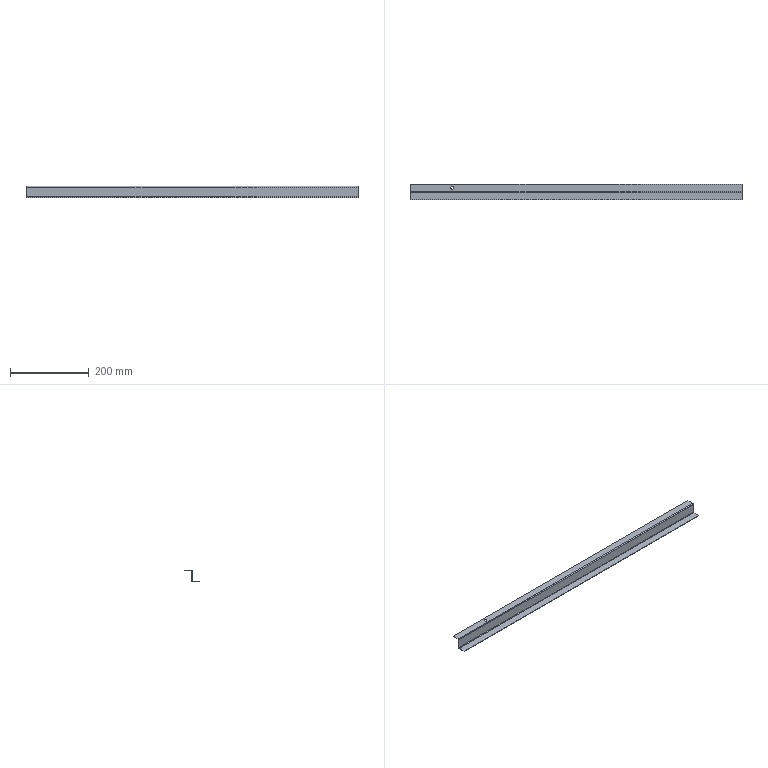Part | SolidWorks | features EdgeFlange 2, FlatPattern 1, HoleWzd 1, SMBaseFlange 1, SheetMetal 1 | 1 solid | 24 faces | box 843 x 38.8 x 28.5 mm | volume 65431 mm3 | plane 18 | cylinder 6 | commonest cylinder face diameters 2 x2 4.4 x2 7 x2
STEP:
#1=CARTESIAN_POINT('',(-310.891,19.773,26.1));
#2=VERTEX_POINT('',#1);
#3=CARTESIAN_POINT('',(-317.891,19.773,26.1));
#4=VERTEX_POINT('',#3);
#5=CARTESIAN_POINT('',(-314.391,19.773,26.1));
#6=DIRECTION('',(0.,0.,-1.));
#7=DIRECTION('',(-1.,0.,0.));
#8=AXIS2_PLACEMENT_3D('',#5,#6,#7);
#9=CIRCLE('',#8,3.5);
#10=EDGE_CURVE('',#2,#4,#9,.T.);
#11=ORIENTED_EDGE('',*,*,#10,.T.);
#12=CARTESIAN_POINT('',(-317.891,19.773,27.3));
#13=VERTEX_POINT('',#12);
#14=CARTESIAN_POINT('',(-317.891,19.773,27.3));
#15=DIRECTION('',(0.,0.,1.));
#16=VECTOR('',#15,1000.);
#17=LINE('',#14,#16);
#18=EDGE_CURVE('',#4,#13,#17,.T.);
#19=ORIENTED_EDGE('',*,*,#18,.T.);
#20=CARTESIAN_POINT('',(-310.891,19.773,27.3));
#21=VERTEX_POINT('',#20);
#22=CARTESIAN_POINT('',(-314.391,19.773,27.3));
#23=DIRECTION('',(0.,0.,1.));
#24=DIRECTION('',(1.,0.,0.));
#25=AXIS2_PLACEMENT_3D('',#22,#23,#24);
#26=CIRCLE('',#25,3.5);
#27=EDGE_CURVE('',#13,#21,#26,.T.);
#28=ORIENTED_EDGE('',*,*,#27,.T.);
#29=CARTESIAN_POINT('',(-310.891,19.773,27.3));
#30=DIRECTION('',(0.,0.,1.));
#31=VECTOR('',#30,1000.);
#32=LINE('',#29,#31);
#33=EDGE_CURVE('',#2,#21,#32,.T.);
#34=ORIENTED_EDGE('',*,*,#33,.F.);
#35=EDGE_LOOP('',(#11,#19,#28,#34));
#36=FACE_OUTER_BOUND('',#35,.T.);
#37=CARTESIAN_POINT('',(-314.391,19.773,27.3));
#38=DIRECTION('',(0.,0.,1.));
#39=DIRECTION('',(1.,0.,0.));
#40=AXIS2_PLACEMENT_3D('',#37,#38,#39);
#41=CYLINDRICAL_SURFACE('',#40,3.5);
#42=ADVANCED_FACE('',(#36),#41,.F.);
#43=CARTESIAN_POINT('',(421.5,10.,25.1));
#44=VERTEX_POINT('',#43);
#45=CARTESIAN_POINT('',(421.5,8.8,25.1));
#46=VERTEX_POINT('',#45);
#47=CARTESIAN_POINT('',(421.5,10.,25.1));
#48=DIRECTION('',(0.,-1.,0.));
#49=VECTOR('',#48,1000.);
#50=LINE('',#47,#49);
#51=EDGE_CURVE('',#44,#46,#50,.T.);
#52=ORIENTED_EDGE('',*,*,#51,.T.);
#53=CARTESIAN_POINT('',(421.5,8.8,1.));
#54=VERTEX_POINT('',#53);
#55=CARTESIAN_POINT('',(421.5,8.8,0.));
#56=DIRECTION('',(0.,0.,-1.));
#57=VECTOR('',#56,1000.);
#58=LINE('',#55,#57);
#59=EDGE_CURVE('',#46,#54,#58,.T.);
#60=ORIENTED_EDGE('',*,*,#59,.T.);
#61=CARTESIAN_POINT('',(421.5,10.,1.));
#62=VERTEX_POINT('',#61);
#63=CARTESIAN_POINT('',(421.5,10.,1.));
#64=DIRECTION('',(0.,1.,0.));
#65=VECTOR('',#64,1000.);
#66=LINE('',#63,#65);
#67=EDGE_CURVE('',#54,#62,#66,.T.);
#68=ORIENTED_EDGE('',*,*,#67,.T.);
#69=CARTESIAN_POINT('',(421.5,10.,0.));
#70=DIRECTION('',(0.,0.,-1.));
#71=VECTOR('',#70,1000.);
#72=LINE('',#69,#71);
#73=EDGE_CURVE('',#44,#62,#72,.T.);
#74=ORIENTED_EDGE('',*,*,#73,.F.);
#75=EDGE_LOOP('',(#52,#60,#68,#74));
#76=FACE_OUTER_BOUND('',#75,.T.);
#77=CARTESIAN_POINT('',(421.5,10.,0.));
#78=DIRECTION('',(-1.,0.,0.));
#79=DIRECTION('',(0.,0.,1.));
#80=AXIS2_PLACEMENT_3D('',#77,#78,#79);
#81=PLANE('',#80);
#82=ADVANCED_FACE('',(#76),#81,.F.);
#83=CARTESIAN_POINT('',(-421.5,10.,25.1));
#84=VERTEX_POINT('',#83);
#85=CARTESIAN_POINT('',(-421.5,8.8,25.1));
#86=VERTEX_POINT('',#85);
#87=CARTESIAN_POINT('',(-421.5,10.,25.1));
#88=DIRECTION('',(0.,-1.,0.));
#89=VECTOR('',#88,1000.);
#90=LINE('',#87,#89);
#91=EDGE_CURVE('',#84,#86,#90,.T.);
#92=ORIENTED_EDGE('',*,*,#91,.F.);
#93=CARTESIAN_POINT('',(-421.5,10.,1.));
#94=VERTEX_POINT('',#93);
#95=CARTESIAN_POINT('',(-421.5,10.,0.));
#96=DIRECTION('',(0.,0.,1.));
#97=VECTOR('',#96,1000.);
#98=LINE('',#95,#97);
#99=EDGE_CURVE('',#94,#84,#98,.T.);
#100=ORIENTED_EDGE('',*,*,#99,.F.);
#101=CARTESIAN_POINT('',(-421.5,8.8,1.));
#102=VERTEX_POINT('',#101);
#103=CARTESIAN_POINT('',(-421.5,8.8,1.));
#104=DIRECTION('',(0.,1.,0.));
#105=VECTOR('',#104,1000.);
#106=LINE('',#103,#105);
#107=EDGE_CURVE('',#102,#94,#106,.T.);
#108=ORIENTED_EDGE('',*,*,#107,.F.);
#109=CARTESIAN_POINT('',(-421.5,8.8,27.3));
#110=DIRECTION('',(0.,0.,1.));
#111=VECTOR('',#110,1000.);
#112=LINE('',#109,#111);
#113=EDGE_CURVE('',#102,#86,#112,.T.);
#114=ORIENTED_EDGE('',*,*,#113,.T.);
#115=EDGE_LOOP('',(#92,#100,#108,#114));
#116=FACE_OUTER_BOUND('',#115,.T.);
#117=CARTESIAN_POINT('',(-421.5,10.,27.3));
#118=DIRECTION('',(1.,0.,0.));
#119=DIRECTION('',(0.,0.,-1.));
#120=AXIS2_PLACEMENT_3D('',#117,#118,#119);
#121=PLANE('',#120);
#122=ADVANCED_FACE('',(#116),#121,.F.);
#123=CARTESIAN_POINT('',(421.5,10.,25.1));
#124=DIRECTION('',(-1.,0.,0.));
#125=VECTOR('',#124,1000.);
#126=LINE('',#123,#125);
#127=EDGE_CURVE('',#44,#84,#126,.T.);
#128=ORIENTED_EDGE('',*,*,#127,.F.);
#129=ORIENTED_EDGE('',*,*,#73,.T.);
#130=CARTESIAN_POINT('',(421.5,10.,1.));
#131=DIRECTION('',(1.,0.,0.));
#132=VECTOR('',#131,1000.);
#133=LINE('',#130,#132);
#134=EDGE_CURVE('',#94,#62,#133,.T.);
#135=ORIENTED_EDGE('',*,*,#134,.F.);
#136=ORIENTED_EDGE('',*,*,#99,.T.);
#137=EDGE_LOOP('',(#128,#129,#135,#136));
#138=FACE_OUTER_BOUND('',#137,.T.);
#139=CARTESIAN_POINT('',(0.,10.,0.));
#140=DIRECTION('',(0.,-1.,0.));
#141=DIRECTION('',(0.,0.,-1.));
#142=AXIS2_PLACEMENT_3D('',#139,#140,#141);
#143=PLANE('',#142);
#144=ADVANCED_FACE('',(#138),#143,.F.);
#145=ORIENTED_EDGE('',*,*,#59,.F.);
#146=CARTESIAN_POINT('',(421.5,8.8,25.1));
#147=DIRECTION('',(-1.,0.,0.));
#148=VECTOR('',#147,1000.);
#149=LINE('',#146,#148);
#150=EDGE_CURVE('',#46,#86,#149,.T.);
#151=ORIENTED_EDGE('',*,*,#150,.T.);
#152=ORIENTED_EDGE('',*,*,#113,.F.);
#153=CARTESIAN_POINT('',(421.5,8.8,1.));
#154=DIRECTION('',(-1.,0.,0.));
#155=VECTOR('',#154,1000.);
#156=LINE('',#153,#155);
#157=EDGE_CURVE('',#54,#102,#156,.T.);
#158=ORIENTED_EDGE('',*,*,#157,.F.);
#159=EDGE_LOOP('',(#145,#151,#152,#158));
#160=FACE_OUTER_BOUND('',#159,.T.);
#161=CARTESIAN_POINT('',(0.,8.8,0.));
#162=DIRECTION('',(0.,-1.,0.));
#163=DIRECTION('',(0.,0.,-1.));
#164=AXIS2_PLACEMENT_3D('',#161,#162,#163);
#165=PLANE('',#164);
#166=ADVANCED_FACE('',(#160),#165,.T.);
#167=CARTESIAN_POINT('',(-421.5,7.8,0.));
#168=VERTEX_POINT('',#167);
#169=CARTESIAN_POINT('',(-421.5,-10.,0.));
#170=VERTEX_POINT('',#169);
#171=CARTESIAN_POINT('',(-421.5,10.,0.));
#172=DIRECTION('',(0.,-1.,0.));
#173=VECTOR('',#172,1000.);
#174=LINE('',#171,#173);
#175=EDGE_CURVE('',#168,#170,#174,.T.);
#176=ORIENTED_EDGE('',*,*,#175,.F.);
#177=CARTESIAN_POINT('',(-421.5,7.8,-1.2));
#178=VERTEX_POINT('',#177);
#179=CARTESIAN_POINT('',(-421.5,7.8,0.));
#180=DIRECTION('',(0.,0.,-1.));
#181=VECTOR('',#180,1000.);
#182=LINE('',#179,#181);
#183=EDGE_CURVE('',#168,#178,#182,.T.);
#184=ORIENTED_EDGE('',*,*,#183,.T.);
#185=CARTESIAN_POINT('',(-421.5,-10.,-1.2));
#186=VERTEX_POINT('',#185);
#187=CARTESIAN_POINT('',(-421.5,10.,-1.2));
#188=DIRECTION('',(0.,-1.,0.));
#189=VECTOR('',#188,1000.);
#190=LINE('',#187,#189);
#191=EDGE_CURVE('',#178,#186,#190,.T.);
#192=ORIENTED_EDGE('',*,*,#191,.T.);
#193=CARTESIAN_POINT('',(-421.5,-10.,-1.2));
#194=DIRECTION('',(0.,0.,1.));
#195=VECTOR('',#194,1000.);
#196=LINE('',#193,#195);
#197=EDGE_CURVE('',#186,#170,#196,.T.);
#198=ORIENTED_EDGE('',*,*,#197,.T.);
#199=EDGE_LOOP('',(#176,#184,#192,#198));
#200=FACE_OUTER_BOUND('',#199,.T.);
#201=CARTESIAN_POINT('',(-421.5,10.,-1.2));
#202=DIRECTION('',(-1.,0.,0.));
#203=DIRECTION('',(0.,0.,1.));
#204=AXIS2_PLACEMENT_3D('',#201,#202,#203);
#205=PLANE('',#204);
#206=ADVANCED_FACE('',(#200),#205,.T.);
#207=CARTESIAN_POINT('',(421.5,7.8,-1.2));
#208=VERTEX_POINT('',#207);
#209=CARTESIAN_POINT('',(-421.5,7.8,-1.2));
#210=DIRECTION('',(1.,0.,0.));
#211=VECTOR('',#210,1000.);
#212=LINE('',#209,#211);
#213=EDGE_CURVE('',#178,#208,#212,.T.);
#214=ORIENTED_EDGE('',*,*,#213,.T.);
#215=CARTESIAN_POINT('',(421.5,-10.,-1.2));
#216=VERTEX_POINT('',#215);
#217=CARTESIAN_POINT('',(421.5,10.,-1.2));
#218=DIRECTION('',(0.,1.,0.));
#219=VECTOR('',#218,1000.);
#220=LINE('',#217,#219);
#221=EDGE_CURVE('',#216,#208,#220,.T.);
#222=ORIENTED_EDGE('',*,*,#221,.F.);
#223=CARTESIAN_POINT('',(-421.5,-10.,-1.2));
#224=DIRECTION('',(1.,0.,0.));
#225=VECTOR('',#224,1000.);
#226=LINE('',#223,#225);
#227=EDGE_CURVE('',#186,#216,#226,.T.);
#228=ORIENTED_EDGE('',*,*,#227,.F.);
#229=ORIENTED_EDGE('',*,*,#191,.F.);
#230=EDGE_LOOP('',(#214,#222,#228,#229));
#231=FACE_OUTER_BOUND('',#230,.T.);
#232=CARTESIAN_POINT('',(0.,0.,-1.2));
#233=DIRECTION('',(0.,0.,1.));
#234=DIRECTION('',(1.,0.,0.));
#235=AXIS2_PLACEMENT_3D('',#232,#233,#234);
#236=PLANE('',#235);
#237=ADVANCED_FACE('',(#231),#236,.F.);
#238=CARTESIAN_POINT('',(421.5,-10.,0.));
#239=VERTEX_POINT('',#238);
#240=CARTESIAN_POINT('',(421.5,7.8,0.));
#241=VERTEX_POINT('',#240);
#242=CARTESIAN_POINT('',(421.5,10.,0.));
#243=DIRECTION('',(0.,1.,0.));
#244=VECTOR('',#243,1000.);
#245=LINE('',#242,#244);
#246=EDGE_CURVE('',#239,#241,#245,.T.);
#247=ORIENTED_EDGE('',*,*,#246,.T.);
#248=CARTESIAN_POINT('',(-421.5,7.8,0.));
#249=DIRECTION('',(1.,0.,0.));
#250=VECTOR('',#249,1000.);
#251=LINE('',#248,#250);
#252=EDGE_CURVE('',#168,#241,#251,.T.);
#253=ORIENTED_EDGE('',*,*,#252,.F.);
#254=ORIENTED_EDGE('',*,*,#175,.T.);
#255=CARTESIAN_POINT('',(-421.5,-10.,0.));
#256=DIRECTION('',(1.,0.,0.));
#257=VECTOR('',#256,1000.);
#258=LINE('',#255,#257);
#259=EDGE_CURVE('',#170,#239,#258,.T.);
#260=ORIENTED_EDGE('',*,*,#259,.T.);
#261=EDGE_LOOP('',(#247,#253,#254,#260));
#262=FACE_OUTER_BOUND('',#261,.T.);
#263=CARTESIAN_POINT('',(0.,0.,0.));
#264=DIRECTION('',(0.,0.,1.));
#265=DIRECTION('',(1.,0.,0.));
#266=AXIS2_PLACEMENT_3D('',#263,#264,#265);
#267=PLANE('',#266);
#268=ADVANCED_FACE('',(#262),#267,.T.);
#269=CARTESIAN_POINT('',(421.5,7.8,0.));
#270=DIRECTION('',(0.,0.,-1.));
#271=VECTOR('',#270,1000.);
#272=LINE('',#269,#271);
#273=EDGE_CURVE('',#241,#208,#272,.T.);
#274=ORIENTED_EDGE('',*,*,#273,.F.);
#275=ORIENTED_EDGE('',*,*,#246,.F.);
#276=CARTESIAN_POINT('',(421.5,-10.,-1.2));
#277=DIRECTION('',(0.,0.,1.));
#278=VECTOR('',#277,1000.);
#279=LINE('',#276,#278);
#280=EDGE_CURVE('',#216,#239,#279,.T.);
#281=ORIENTED_EDGE('',*,*,#280,.F.);
#282=ORIENTED_EDGE('',*,*,#221,.T.);
#283=EDGE_LOOP('',(#274,#275,#281,#282));
#284=FACE_OUTER_BOUND('',#283,.T.);
#285=CARTESIAN_POINT('',(421.5,10.,-1.2));
#286=DIRECTION('',(1.,0.,0.));
#287=DIRECTION('',(0.,0.,-1.));
#288=AXIS2_PLACEMENT_3D('',#285,#286,#287);
#289=PLANE('',#288);
#290=ADVANCED_FACE('',(#284),#289,.T.);
#291=ORIENTED_EDGE('',*,*,#259,.F.);
#292=ORIENTED_EDGE('',*,*,#197,.F.);
#293=ORIENTED_EDGE('',*,*,#227,.T.);
#294=ORIENTED_EDGE('',*,*,#280,.T.);
#295=EDGE_LOOP('',(#291,#292,#293,#294));
#296=FACE_OUTER_BOUND('',#295,.T.);
#297=CARTESIAN_POINT('',(-421.5,-10.,-1.2));
#298=DIRECTION('',(0.,-1.,0.));
#299=DIRECTION('',(0.,0.,-1.));
#300=AXIS2_PLACEMENT_3D('',#297,#298,#299);
#301=PLANE('',#300);
#302=ADVANCED_FACE('',(#296),#301,.T.);
#303=ORIENTED_EDGE('',*,*,#67,.F.);
#304=CARTESIAN_POINT('',(421.5,7.8,1.));
#305=DIRECTION('',(1.,0.,0.));
#306=DIRECTION('',(0.,0.,1.));
#307=AXIS2_PLACEMENT_3D('',#304,#305,#306);
#308=CIRCLE('',#307,1.);
#309=EDGE_CURVE('',#241,#54,#308,.T.);
#310=ORIENTED_EDGE('',*,*,#309,.F.);
#311=ORIENTED_EDGE('',*,*,#273,.T.);
#312=CARTESIAN_POINT('',(421.5,7.8,1.));
#313=DIRECTION('',(1.,0.,0.));
#314=DIRECTION('',(0.,0.,1.));
#315=AXIS2_PLACEMENT_3D('',#312,#313,#314);
#316=CIRCLE('',#315,2.2);
#317=EDGE_CURVE('',#208,#62,#316,.T.);
#318=ORIENTED_EDGE('',*,*,#317,.T.);
#319=EDGE_LOOP('',(#303,#310,#311,#318));
#320=FACE_OUTER_BOUND('',#319,.T.);
#321=CARTESIAN_POINT('',(421.5,7.8,1.));
#322=DIRECTION('',(1.,0.,0.));
#323=DIRECTION('',(0.,0.,-1.));
#324=AXIS2_PLACEMENT_3D('',#321,#322,#323);
#325=PLANE('',#324);
#326=ADVANCED_FACE('',(#320),#325,.T.);
#327=CARTESIAN_POINT('',(-421.5,7.8,1.));
#328=DIRECTION('',(-1.,0.,0.));
#329=DIRECTION('',(0.,0.,1.));
#330=AXIS2_PLACEMENT_3D('',#327,#328,#329);
#331=CIRCLE('',#330,1.);
#332=EDGE_CURVE('',#102,#168,#331,.T.);
#333=ORIENTED_EDGE('',*,*,#332,.F.);
#334=ORIENTED_EDGE('',*,*,#107,.T.);
#335=CARTESIAN_POINT('',(-421.5,7.8,1.));
#336=DIRECTION('',(-1.,0.,0.));
#337=DIRECTION('',(0.,0.,1.));
#338=AXIS2_PLACEMENT_3D('',#335,#336,#337);
#339=CIRCLE('',#338,2.2);
#340=EDGE_CURVE('',#94,#178,#339,.T.);
#341=ORIENTED_EDGE('',*,*,#340,.T.);
#342=ORIENTED_EDGE('',*,*,#183,.F.);
#343=EDGE_LOOP('',(#333,#334,#341,#342));
#344=FACE_OUTER_BOUND('',#343,.T.);
#345=CARTESIAN_POINT('',(-421.5,7.8,1.));
#346=DIRECTION('',(1.,0.,0.));
#347=DIRECTION('',(0.,0.,-1.));
#348=AXIS2_PLACEMENT_3D('',#345,#346,#347);
#349=PLANE('',#348);
#350=ADVANCED_FACE('',(#344),#349,.F.);
#351=ORIENTED_EDGE('',*,*,#213,.F.);
#352=ORIENTED_EDGE('',*,*,#340,.F.);
#353=ORIENTED_EDGE('',*,*,#134,.T.);
#354=ORIENTED_EDGE('',*,*,#317,.F.);
#355=EDGE_LOOP('',(#351,#352,#353,#354));
#356=FACE_OUTER_BOUND('',#355,.T.);
#357=CARTESIAN_POINT('',(-421.5,7.8,1.));
#358=DIRECTION('',(-1.,0.,0.));
#359=DIRECTION('',(0.,1.,0.));
#360=AXIS2_PLACEMENT_3D('',#357,#358,#359);
#361=CYLINDRICAL_SURFACE('',#360,2.2);
#362=ADVANCED_FACE('',(#356),#361,.T.);
#363=ORIENTED_EDGE('',*,*,#252,.T.);
#364=ORIENTED_EDGE('',*,*,#309,.T.);
#365=ORIENTED_EDGE('',*,*,#157,.T.);
#366=ORIENTED_EDGE('',*,*,#332,.T.);
#367=EDGE_LOOP('',(#363,#364,#365,#366));
#368=FACE_OUTER_BOUND('',#367,.T.);
#369=CARTESIAN_POINT('',(-421.5,7.8,1.));
#370=DIRECTION('',(-1.,0.,0.));
#371=DIRECTION('',(0.,1.,0.));
#372=AXIS2_PLACEMENT_3D('',#369,#370,#371);
#373=CYLINDRICAL_SURFACE('',#372,1.);
#374=ADVANCED_FACE('',(#368),#373,.F.);
#375=CARTESIAN_POINT('',(-421.5,11.,26.1));
#376=VERTEX_POINT('',#375);
#377=CARTESIAN_POINT('',(-421.5,11.,27.3));
#378=VERTEX_POINT('',#377);
#379=CARTESIAN_POINT('',(-421.5,11.,27.3));
#380=DIRECTION('',(0.,0.,1.));
#381=VECTOR('',#380,1000.);
#382=LINE('',#379,#381);
#383=EDGE_CURVE('',#376,#378,#382,.T.);
#384=ORIENTED_EDGE('',*,*,#383,.F.);
#385=CARTESIAN_POINT('',(-421.5,11.,25.1));
#386=DIRECTION('',(-1.,0.,0.));
#387=DIRECTION('',(0.,0.,-1.));
#388=AXIS2_PLACEMENT_3D('',#385,#386,#387);
#389=CIRCLE('',#388,1.);
#390=EDGE_CURVE('',#84,#376,#389,.T.);
#391=ORIENTED_EDGE('',*,*,#390,.F.);
#392=ORIENTED_EDGE('',*,*,#91,.T.);
#393=CARTESIAN_POINT('',(-421.5,11.,25.1));
#394=DIRECTION('',(-1.,0.,0.));
#395=DIRECTION('',(0.,0.,-1.));
#396=AXIS2_PLACEMENT_3D('',#393,#394,#395);
#397=CIRCLE('',#396,2.2);
#398=EDGE_CURVE('',#86,#378,#397,.T.);
#399=ORIENTED_EDGE('',*,*,#398,.T.);
#400=EDGE_LOOP('',(#384,#391,#392,#399));
#401=FACE_OUTER_BOUND('',#400,.T.);
#402=CARTESIAN_POINT('',(-421.5,11.,25.1));
#403=DIRECTION('',(-1.,0.,0.));
#404=DIRECTION('',(0.,0.,1.));
#405=AXIS2_PLACEMENT_3D('',#402,#403,#404);
#406=PLANE('',#405);
#407=ADVANCED_FACE('',(#401),#406,.T.);
#408=CARTESIAN_POINT('',(421.5,11.,26.1));
#409=VERTEX_POINT('',#408);
#410=CARTESIAN_POINT('',(421.5,11.,25.1));
#411=DIRECTION('',(1.,0.,0.));
#412=DIRECTION('',(0.,0.,-1.));
#413=AXIS2_PLACEMENT_3D('',#410,#411,#412);
#414=CIRCLE('',#413,1.);
#415=EDGE_CURVE('',#409,#44,#414,.T.);
#416=ORIENTED_EDGE('',*,*,#415,.F.);
#417=CARTESIAN_POINT('',(421.5,11.,27.3));
#418=VERTEX_POINT('',#417);
#419=CARTESIAN_POINT('',(421.5,11.,26.1));
#420=DIRECTION('',(0.,0.,1.));
#421=VECTOR('',#420,1000.);
#422=LINE('',#419,#421);
#423=EDGE_CURVE('',#409,#418,#422,.T.);
#424=ORIENTED_EDGE('',*,*,#423,.T.);
#425=CARTESIAN_POINT('',(421.5,11.,25.1));
#426=DIRECTION('',(1.,0.,0.));
#427=DIRECTION('',(0.,0.,-1.));
#428=AXIS2_PLACEMENT_3D('',#425,#426,#427);
#429=CIRCLE('',#428,2.2);
#430=EDGE_CURVE('',#418,#46,#429,.T.);
#431=ORIENTED_EDGE('',*,*,#430,.T.);
#432=ORIENTED_EDGE('',*,*,#51,.F.);
#433=EDGE_LOOP('',(#416,#424,#431,#432));
#434=FACE_OUTER_BOUND('',#433,.T.);
#435=CARTESIAN_POINT('',(421.5,11.,25.1));
#436=DIRECTION('',(-1.,0.,0.));
#437=DIRECTION('',(0.,0.,1.));
#438=AXIS2_PLACEMENT_3D('',#435,#436,#437);
#439=PLANE('',#438);
#440=ADVANCED_FACE('',(#434),#439,.F.);
#441=ORIENTED_EDGE('',*,*,#150,.F.);
#442=ORIENTED_EDGE('',*,*,#430,.F.);
#443=CARTESIAN_POINT('',(-421.5,11.,27.3));
#444=DIRECTION('',(-1.,0.,0.));
#445=VECTOR('',#444,1000.);
#446=LINE('',#443,#445);
#447=EDGE_CURVE('',#418,#378,#446,.T.);
#448=ORIENTED_EDGE('',*,*,#447,.T.);
#449=ORIENTED_EDGE('',*,*,#398,.F.);
#450=EDGE_LOOP('',(#441,#442,#448,#449));
#451=FACE_OUTER_BOUND('',#450,.T.);
#452=CARTESIAN_POINT('',(421.5,11.,25.1));
#453=DIRECTION('',(1.,0.,0.));
#454=DIRECTION('',(0.,0.,1.));
#455=AXIS2_PLACEMENT_3D('',#452,#453,#454);
#456=CYLINDRICAL_SURFACE('',#455,2.2);
#457=ADVANCED_FACE('',(#451),#456,.T.);
#458=ORIENTED_EDGE('',*,*,#127,.T.);
#459=ORIENTED_EDGE('',*,*,#390,.T.);
#460=CARTESIAN_POINT('',(-421.5,11.,26.1));
#461=DIRECTION('',(1.,0.,0.));
#462=VECTOR('',#461,1000.);
#463=LINE('',#460,#462);
#464=EDGE_CURVE('',#376,#409,#463,.T.);
#465=ORIENTED_EDGE('',*,*,#464,.T.);
#466=ORIENTED_EDGE('',*,*,#415,.T.);
#467=EDGE_LOOP('',(#458,#459,#465,#466));
#468=FACE_OUTER_BOUND('',#467,.T.);
#469=CARTESIAN_POINT('',(421.5,11.,25.1));
#470=DIRECTION('',(1.,0.,0.));
#471=DIRECTION('',(0.,0.,1.));
#472=AXIS2_PLACEMENT_3D('',#469,#470,#471);
#473=CYLINDRICAL_SURFACE('',#472,1.);
#474=ADVANCED_FACE('',(#468),#473,.F.);
#475=ORIENTED_EDGE('',*,*,#383,.T.);
#476=CARTESIAN_POINT('',(-421.5,28.8,27.3));
#477=VERTEX_POINT('',#476);
#478=CARTESIAN_POINT('',(-421.5,0.,27.3));
#479=DIRECTION('',(0.,-1.,0.));
#480=VECTOR('',#479,1000.);
#481=LINE('',#478,#480);
#482=EDGE_CURVE('',#477,#378,#481,.T.);
#483=ORIENTED_EDGE('',*,*,#482,.F.);
#484=CARTESIAN_POINT('',(-421.5,28.8,26.1));
#485=VERTEX_POINT('',#484);
#486=CARTESIAN_POINT('',(-421.5,28.8,27.3));
#487=DIRECTION('',(0.,0.,-1.));
#488=VECTOR('',#487,1000.);
#489=LINE('',#486,#488);
#490=EDGE_CURVE('',#477,#485,#489,.T.);
#491=ORIENTED_EDGE('',*,*,#490,.T.);
#492=CARTESIAN_POINT('',(-421.5,10.,26.1));
#493=DIRECTION('',(0.,-1.,0.));
#494=VECTOR('',#493,1000.);
#495=LINE('',#492,#494);
#496=EDGE_CURVE('',#485,#376,#495,.T.);
#497=ORIENTED_EDGE('',*,*,#496,.T.);
#498=EDGE_LOOP('',(#475,#483,#491,#497));
#499=FACE_OUTER_BOUND('',#498,.T.);
#500=CARTESIAN_POINT('',(-421.5,10.,27.3));
#501=DIRECTION('',(1.,0.,0.));
#502=DIRECTION('',(0.,0.,-1.));
#503=AXIS2_PLACEMENT_3D('',#500,#501,#502);
#504=PLANE('',#503);
#505=ADVANCED_FACE('',(#499),#504,.F.);
#506=ORIENTED_EDGE('',*,*,#423,.F.);
#507=CARTESIAN_POINT('',(421.5,28.8,26.1));
#508=VERTEX_POINT('',#507);
#509=CARTESIAN_POINT('',(421.5,28.8,26.1));
#510=DIRECTION('',(0.,1.,0.));
#511=VECTOR('',#510,1000.);
#512=LINE('',#509,#511);
#513=EDGE_CURVE('',#409,#508,#512,.T.);
#514=ORIENTED_EDGE('',*,*,#513,.T.);
#515=CARTESIAN_POINT('',(421.5,28.8,27.3));
#516=VERTEX_POINT('',#515);
#517=CARTESIAN_POINT('',(421.5,28.8,27.3));
#518=DIRECTION('',(0.,0.,-1.));
#519=VECTOR('',#518,1000.);
#520=LINE('',#517,#519);
#521=EDGE_CURVE('',#516,#508,#520,.T.);
#522=ORIENTED_EDGE('',*,*,#521,.F.);
#523=CARTESIAN_POINT('',(421.5,0.,27.3));
#524=DIRECTION('',(0.,1.,0.));
#525=VECTOR('',#524,1000.);
#526=LINE('',#523,#525);
#527=EDGE_CURVE('',#418,#516,#526,.T.);
#528=ORIENTED_EDGE('',*,*,#527,.F.);
#529=EDGE_LOOP('',(#506,#514,#522,#528));
#530=FACE_OUTER_BOUND('',#529,.T.);
#531=CARTESIAN_POINT('',(421.5,28.8,27.3));
#532=DIRECTION('',(-1.,0.,0.));
#533=DIRECTION('',(0.,-1.,0.));
#534=AXIS2_PLACEMENT_3D('',#531,#532,#533);
#535=PLANE('',#534);
#536=ADVANCED_FACE('',(#530),#535,.F.);
#537=CARTESIAN_POINT('',(-314.391,19.773,27.3));
#538=DIRECTION('',(0.,0.,1.));
#539=DIRECTION('',(1.,0.,0.));
#540=AXIS2_PLACEMENT_3D('',#537,#538,#539);
#541=CIRCLE('',#540,3.5);
#542=EDGE_CURVE('',#21,#13,#541,.T.);
#543=ORIENTED_EDGE('',*,*,#542,.F.);
#544=ORIENTED_EDGE('',*,*,#27,.F.);
#545=EDGE_LOOP('',(#543,#544));
#546=FACE_BOUND('',#545,.T.);
#547=ORIENTED_EDGE('',*,*,#447,.F.);
#548=ORIENTED_EDGE('',*,*,#527,.T.);
#549=CARTESIAN_POINT('',(0.,28.8,27.3));
#550=DIRECTION('',(-1.,0.,0.));
#551=VECTOR('',#550,1000.);
#552=LINE('',#549,#551);
#553=EDGE_CURVE('',#516,#477,#552,.T.);
#554=ORIENTED_EDGE('',*,*,#553,.T.);
#555=ORIENTED_EDGE('',*,*,#482,.T.);
#556=EDGE_LOOP('',(#547,#548,#554,#555));
#557=FACE_OUTER_BOUND('',#556,.T.);
#558=CARTESIAN_POINT('',(0.,0.,27.3));
#559=DIRECTION('',(0.,0.,-1.));
#560=DIRECTION('',(-1.,0.,0.));
#561=AXIS2_PLACEMENT_3D('',#558,#559,#560);
#562=PLANE('',#561);
#563=ADVANCED_FACE('',(#546,#557),#562,.F.);
#564=ORIENTED_EDGE('',*,*,#10,.F.);
#565=CARTESIAN_POINT('',(-314.391,19.773,26.1));
#566=DIRECTION('',(0.,0.,-1.));
#567=DIRECTION('',(-1.,0.,0.));
#568=AXIS2_PLACEMENT_3D('',#565,#566,#567);
#569=CIRCLE('',#568,3.5);
#570=EDGE_CURVE('',#4,#2,#569,.T.);
#571=ORIENTED_EDGE('',*,*,#570,.F.);
#572=EDGE_LOOP('',(#564,#571));
#573=FACE_BOUND('',#572,.T.);
#574=ORIENTED_EDGE('',*,*,#513,.F.);
#575=ORIENTED_EDGE('',*,*,#464,.F.);
#576=ORIENTED_EDGE('',*,*,#496,.F.);
#577=CARTESIAN_POINT('',(-421.5,28.8,26.1));
#578=DIRECTION('',(-1.,0.,0.));
#579=VECTOR('',#578,1000.);
#580=LINE('',#577,#579);
#581=EDGE_CURVE('',#508,#485,#580,.T.);
#582=ORIENTED_EDGE('',*,*,#581,.F.);
#583=EDGE_LOOP('',(#574,#575,#576,#582));
#584=FACE_OUTER_BOUND('',#583,.T.);
#585=CARTESIAN_POINT('',(0.,0.,26.1));
#586=DIRECTION('',(0.,0.,-1.));
#587=DIRECTION('',(-1.,0.,0.));
#588=AXIS2_PLACEMENT_3D('',#585,#586,#587);
#589=PLANE('',#588);
#590=ADVANCED_FACE('',(#573,#584),#589,.T.);
#591=ORIENTED_EDGE('',*,*,#581,.T.);
#592=ORIENTED_EDGE('',*,*,#490,.F.);
#593=ORIENTED_EDGE('',*,*,#553,.F.);
#594=ORIENTED_EDGE('',*,*,#521,.T.);
#595=EDGE_LOOP('',(#591,#592,#593,#594));
#596=FACE_OUTER_BOUND('',#595,.T.);
#597=CARTESIAN_POINT('',(-421.5,28.8,27.3));
#598=DIRECTION('',(0.,-1.,0.));
#599=DIRECTION('',(0.,0.,-1.));
#600=AXIS2_PLACEMENT_3D('',#597,#598,#599);
#601=PLANE('',#600);
#602=ADVANCED_FACE('',(#596),#601,.F.);
#603=ORIENTED_EDGE('',*,*,#18,.F.);
#604=ORIENTED_EDGE('',*,*,#570,.T.);
#605=ORIENTED_EDGE('',*,*,#33,.T.);
#606=ORIENTED_EDGE('',*,*,#542,.T.);
#607=EDGE_LOOP('',(#603,#604,#605,#606));
#608=FACE_OUTER_BOUND('',#607,.T.);
#609=CARTESIAN_POINT('',(-314.391,19.773,27.3));
#610=DIRECTION('',(0.,0.,1.));
#611=DIRECTION('',(1.,0.,0.));
#612=AXIS2_PLACEMENT_3D('',#609,#610,#611);
#613=CYLINDRICAL_SURFACE('',#612,3.5);
#614=ADVANCED_FACE('',(#608),#613,.F.);
#615=CLOSED_SHELL('',(#42,#82,#122,#144,#166,#206,#237,#268,#290,#302,#326,#350,#362,#374,#407,#440,#457,#474,#505,#536,#563,#590,#602,#614));
#616=MANIFOLD_SOLID_BREP('',#615);
#617=CARTESIAN_POINT('',(0.,0.,0.));
#618=DIRECTION('',(0.,0.,1.));
#619=DIRECTION('',(1.,0.,0.));
#620=AXIS2_PLACEMENT_3D('',#617,#618,#619);
#621=(LENGTH_UNIT()NAMED_UNIT(*)SI_UNIT(.MILLI.,.METRE.));
#622=UNCERTAINTY_MEASURE_WITH_UNIT(LENGTH_MEASURE(0.00001),#621,'','');
#623=(NAMED_UNIT(*)PLANE_ANGLE_UNIT()SI_UNIT($,.RADIAN.));
#624=(NAMED_UNIT(*)SI_UNIT($,.STERADIAN.)SOLID_ANGLE_UNIT());
#625=(GEOMETRIC_REPRESENTATION_CONTEXT(3)GLOBAL_UNCERTAINTY_ASSIGNED_CONTEXT((#622))GLOBAL_UNIT_ASSIGNED_CONTEXT((#621,#623,#624))REPRESENTATION_CONTEXT('',''));
#626=ADVANCED_BREP_SHAPE_REPRESENTATION('',(#616,#620),#625);